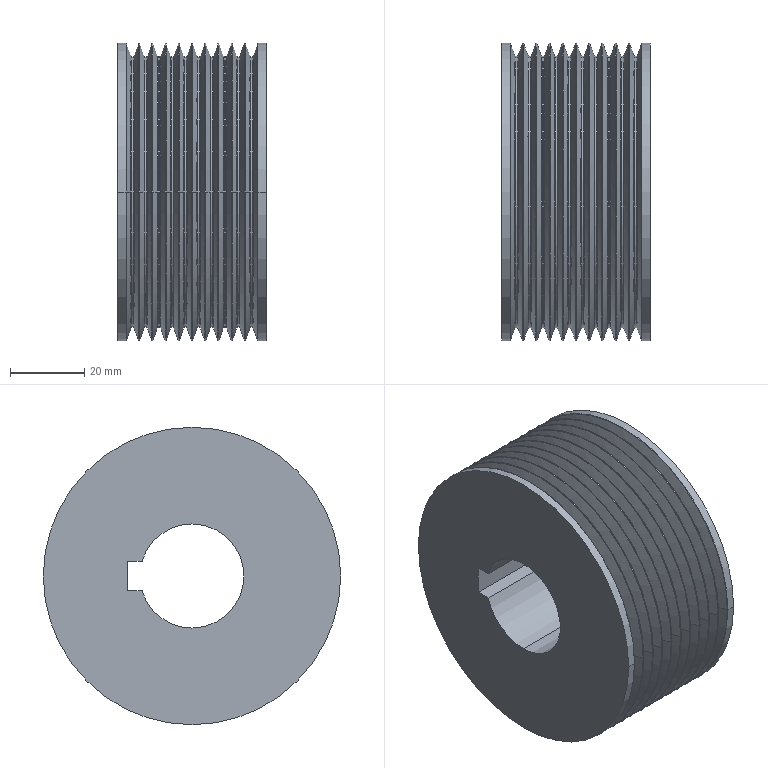Part | SolidWorks | features ICE 1, Revolution 1 | 1 solid | 170 faces | box 39.93 x 80 x 80 mm | volume 157702 mm3 | torus 80 | cylinder 45 | cone 40 | plane 5 | commonest cylinder face diameters 80 x22 73.1 x20 28 x3